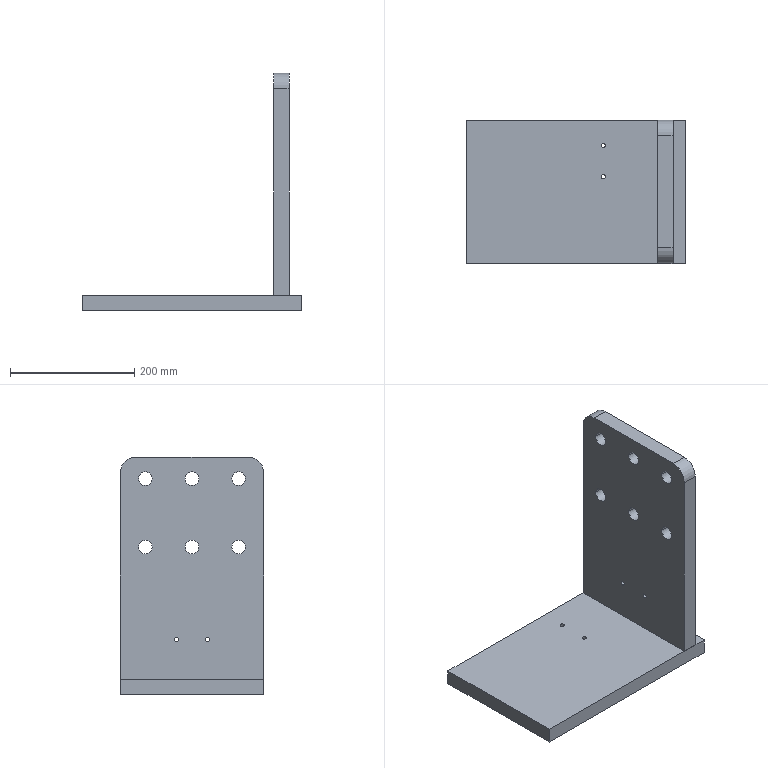Part | STEP file | 2 solids | 34 faces | box 352 x 230 x 382 mm | volume 4009392 mm3 | cylinder 22 | plane 12 | commonest cylinder face diameters 22 x12 6.8 x8 50 x2